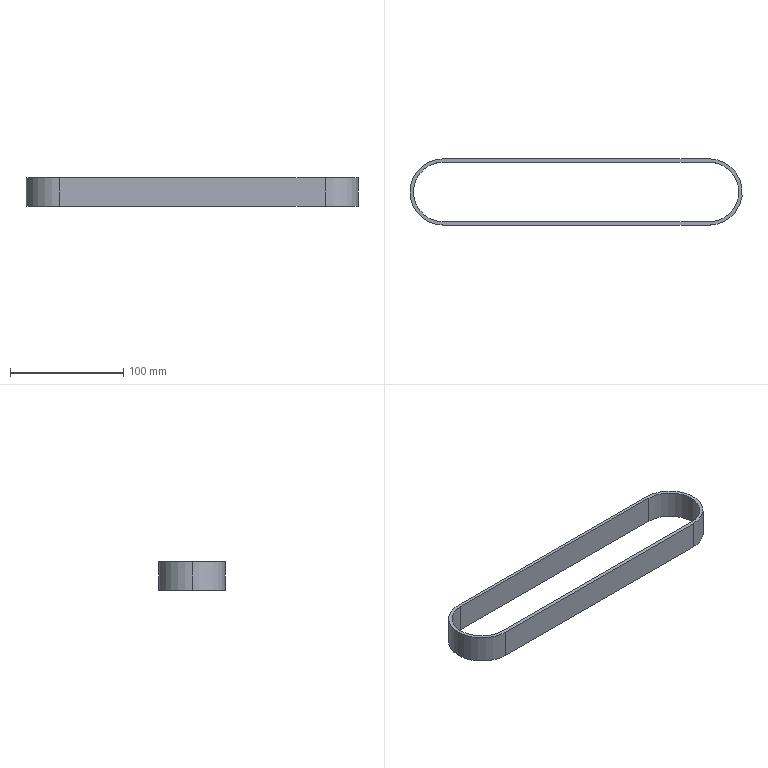Part | SolidWorks | features BeltProfileFeature 1, ExtruThin 1 | 1 solid | 12 faces | box 293.56 x 58.56 x 25 mm | volume 48341 mm3 | cylinder 6 | plane 6 | commonest cylinder face diameters 52.56 x3 58.56 x3
STEP:
#1=CARTESIAN_POINT('',(-235.,26.28,12.5));
#2=VERTEX_POINT('',#1);
#3=CARTESIAN_POINT('',(-261.28,0.,12.5));
#4=VERTEX_POINT('',#3);
#5=CARTESIAN_POINT('',(-235.,0.,12.5));
#6=DIRECTION('',(0.,0.,1.));
#7=DIRECTION('',(-1.,0.,0.));
#8=AXIS2_PLACEMENT_3D('',#5,#6,#7);
#9=CIRCLE('',#8,26.28);
#10=EDGE_CURVE('',#2,#4,#9,.T.);
#11=ORIENTED_EDGE('',*,*,#10,.T.);
#12=CARTESIAN_POINT('',(-261.28,0.,-12.5));
#13=VERTEX_POINT('',#12);
#14=CARTESIAN_POINT('',(-261.28,0.,12.5));
#15=DIRECTION('',(0.,0.,-1.));
#16=VECTOR('',#15,1000.);
#17=LINE('',#14,#16);
#18=EDGE_CURVE('',#4,#13,#17,.T.);
#19=ORIENTED_EDGE('',*,*,#18,.T.);
#20=CARTESIAN_POINT('',(-235.,26.28,-12.5));
#21=VERTEX_POINT('',#20);
#22=CARTESIAN_POINT('',(-235.,0.,-12.5));
#23=DIRECTION('',(0.,0.,1.));
#24=DIRECTION('',(-1.,0.,0.));
#25=AXIS2_PLACEMENT_3D('',#22,#23,#24);
#26=CIRCLE('',#25,26.28);
#27=EDGE_CURVE('',#21,#13,#26,.T.);
#28=ORIENTED_EDGE('',*,*,#27,.F.);
#29=CARTESIAN_POINT('',(-235.,26.28,12.5));
#30=DIRECTION('',(0.,0.,-1.));
#31=VECTOR('',#30,1000.);
#32=LINE('',#29,#31);
#33=EDGE_CURVE('',#2,#21,#32,.T.);
#34=ORIENTED_EDGE('',*,*,#33,.F.);
#35=EDGE_LOOP('',(#11,#19,#28,#34));
#36=FACE_OUTER_BOUND('',#35,.T.);
#37=CARTESIAN_POINT('',(-235.,0.,12.5));
#38=DIRECTION('',(0.,0.,-1.));
#39=DIRECTION('',(-1.,0.,0.));
#40=AXIS2_PLACEMENT_3D('',#37,#38,#39);
#41=CYLINDRICAL_SURFACE('',#40,26.28);
#42=ADVANCED_FACE('',(#36),#41,.F.);
#43=CARTESIAN_POINT('',(-264.28,0.,12.5));
#44=VERTEX_POINT('',#43);
#45=CARTESIAN_POINT('',(-235.,-29.28,12.5));
#46=VERTEX_POINT('',#45);
#47=CARTESIAN_POINT('',(-235.,0.,12.5));
#48=DIRECTION('',(0.,0.,1.));
#49=DIRECTION('',(-1.,0.,0.));
#50=AXIS2_PLACEMENT_3D('',#47,#48,#49);
#51=CIRCLE('',#50,29.28);
#52=EDGE_CURVE('',#44,#46,#51,.T.);
#53=ORIENTED_EDGE('',*,*,#52,.F.);
#54=CARTESIAN_POINT('',(-264.28,0.,-12.5));
#55=VERTEX_POINT('',#54);
#56=CARTESIAN_POINT('',(-264.28,0.,12.5));
#57=DIRECTION('',(0.,0.,-1.));
#58=VECTOR('',#57,1000.);
#59=LINE('',#56,#58);
#60=EDGE_CURVE('',#44,#55,#59,.T.);
#61=ORIENTED_EDGE('',*,*,#60,.T.);
#62=CARTESIAN_POINT('',(-235.,-29.28,-12.5));
#63=VERTEX_POINT('',#62);
#64=CARTESIAN_POINT('',(-235.,0.,-12.5));
#65=DIRECTION('',(0.,0.,1.));
#66=DIRECTION('',(-1.,0.,0.));
#67=AXIS2_PLACEMENT_3D('',#64,#65,#66);
#68=CIRCLE('',#67,29.28);
#69=EDGE_CURVE('',#55,#63,#68,.T.);
#70=ORIENTED_EDGE('',*,*,#69,.T.);
#71=CARTESIAN_POINT('',(-235.,-29.28,12.5));
#72=DIRECTION('',(0.,0.,-1.));
#73=VECTOR('',#72,1000.);
#74=LINE('',#71,#73);
#75=EDGE_CURVE('',#46,#63,#74,.T.);
#76=ORIENTED_EDGE('',*,*,#75,.F.);
#77=EDGE_LOOP('',(#53,#61,#70,#76));
#78=FACE_OUTER_BOUND('',#77,.T.);
#79=CARTESIAN_POINT('',(-235.,0.,12.5));
#80=DIRECTION('',(0.,0.,-1.));
#81=DIRECTION('',(-1.,0.,0.));
#82=AXIS2_PLACEMENT_3D('',#79,#80,#81);
#83=CYLINDRICAL_SURFACE('',#82,29.28);
#84=ADVANCED_FACE('',(#78),#83,.T.);
#85=CARTESIAN_POINT('',(0.,-29.28,12.5));
#86=VERTEX_POINT('',#85);
#87=CARTESIAN_POINT('',(0.,29.28,12.5));
#88=VERTEX_POINT('',#87);
#89=CARTESIAN_POINT('',(0.,0.,12.5));
#90=DIRECTION('',(0.,0.,1.));
#91=DIRECTION('',(-1.,0.,0.));
#92=AXIS2_PLACEMENT_3D('',#89,#90,#91);
#93=CIRCLE('',#92,29.28);
#94=EDGE_CURVE('',#86,#88,#93,.T.);
#95=ORIENTED_EDGE('',*,*,#94,.T.);
#96=CARTESIAN_POINT('',(-235.,29.28,12.5));
#97=VERTEX_POINT('',#96);
#98=CARTESIAN_POINT('',(0.,29.28,12.5));
#99=DIRECTION('',(-1.,0.,0.));
#100=VECTOR('',#99,1000.);
#101=LINE('',#98,#100);
#102=EDGE_CURVE('',#88,#97,#101,.T.);
#103=ORIENTED_EDGE('',*,*,#102,.T.);
#104=CARTESIAN_POINT('',(-235.,0.,12.5));
#105=DIRECTION('',(0.,0.,1.));
#106=DIRECTION('',(-1.,0.,0.));
#107=AXIS2_PLACEMENT_3D('',#104,#105,#106);
#108=CIRCLE('',#107,29.28);
#109=EDGE_CURVE('',#97,#44,#108,.T.);
#110=ORIENTED_EDGE('',*,*,#109,.T.);
#111=ORIENTED_EDGE('',*,*,#52,.T.);
#112=CARTESIAN_POINT('',(0.,-29.28,12.5));
#113=DIRECTION('',(1.,0.,0.));
#114=VECTOR('',#113,1000.);
#115=LINE('',#112,#114);
#116=EDGE_CURVE('',#46,#86,#115,.T.);
#117=ORIENTED_EDGE('',*,*,#116,.T.);
#118=EDGE_LOOP('',(#95,#103,#110,#111,#117));
#119=FACE_OUTER_BOUND('',#118,.T.);
#120=CARTESIAN_POINT('',(0.,-26.28,12.5));
#121=VERTEX_POINT('',#120);
#122=CARTESIAN_POINT('',(0.,26.28,12.5));
#123=VERTEX_POINT('',#122);
#124=CARTESIAN_POINT('',(0.,0.,12.5));
#125=DIRECTION('',(0.,0.,1.));
#126=DIRECTION('',(-1.,0.,0.));
#127=AXIS2_PLACEMENT_3D('',#124,#125,#126);
#128=CIRCLE('',#127,26.28);
#129=EDGE_CURVE('',#121,#123,#128,.T.);
#130=ORIENTED_EDGE('',*,*,#129,.F.);
#131=CARTESIAN_POINT('',(-235.,-26.28,12.5));
#132=VERTEX_POINT('',#131);
#133=CARTESIAN_POINT('',(0.,-26.28,12.5));
#134=DIRECTION('',(1.,0.,0.));
#135=VECTOR('',#134,1000.);
#136=LINE('',#133,#135);
#137=EDGE_CURVE('',#132,#121,#136,.T.);
#138=ORIENTED_EDGE('',*,*,#137,.F.);
#139=CARTESIAN_POINT('',(-235.,0.,12.5));
#140=DIRECTION('',(0.,0.,1.));
#141=DIRECTION('',(-1.,0.,0.));
#142=AXIS2_PLACEMENT_3D('',#139,#140,#141);
#143=CIRCLE('',#142,26.28);
#144=EDGE_CURVE('',#4,#132,#143,.T.);
#145=ORIENTED_EDGE('',*,*,#144,.F.);
#146=ORIENTED_EDGE('',*,*,#10,.F.);
#147=CARTESIAN_POINT('',(-235.,26.28,12.5));
#148=DIRECTION('',(-1.,0.,0.));
#149=VECTOR('',#148,1000.);
#150=LINE('',#147,#149);
#151=EDGE_CURVE('',#123,#2,#150,.T.);
#152=ORIENTED_EDGE('',*,*,#151,.F.);
#153=EDGE_LOOP('',(#130,#138,#145,#146,#152));
#154=FACE_BOUND('',#153,.T.);
#155=CARTESIAN_POINT('',(0.,0.,12.5));
#156=DIRECTION('',(0.,0.,-1.));
#157=DIRECTION('',(-1.,0.,0.));
#158=AXIS2_PLACEMENT_3D('',#155,#156,#157);
#159=PLANE('',#158);
#160=ADVANCED_FACE('',(#119,#154),#159,.F.);
#161=CARTESIAN_POINT('',(0.,-29.28,-12.5));
#162=VERTEX_POINT('',#161);
#163=CARTESIAN_POINT('',(0.,29.28,-12.5));
#164=VERTEX_POINT('',#163);
#165=CARTESIAN_POINT('',(0.,0.,-12.5));
#166=DIRECTION('',(0.,0.,1.));
#167=DIRECTION('',(-1.,0.,0.));
#168=AXIS2_PLACEMENT_3D('',#165,#166,#167);
#169=CIRCLE('',#168,29.28);
#170=EDGE_CURVE('',#162,#164,#169,.T.);
#171=ORIENTED_EDGE('',*,*,#170,.F.);
#172=CARTESIAN_POINT('',(0.,-29.28,-12.5));
#173=DIRECTION('',(1.,0.,0.));
#174=VECTOR('',#173,1000.);
#175=LINE('',#172,#174);
#176=EDGE_CURVE('',#63,#162,#175,.T.);
#177=ORIENTED_EDGE('',*,*,#176,.F.);
#178=ORIENTED_EDGE('',*,*,#69,.F.);
#179=CARTESIAN_POINT('',(-235.,29.28,-12.5));
#180=VERTEX_POINT('',#179);
#181=CARTESIAN_POINT('',(-235.,0.,-12.5));
#182=DIRECTION('',(0.,0.,1.));
#183=DIRECTION('',(-1.,0.,0.));
#184=AXIS2_PLACEMENT_3D('',#181,#182,#183);
#185=CIRCLE('',#184,29.28);
#186=EDGE_CURVE('',#180,#55,#185,.T.);
#187=ORIENTED_EDGE('',*,*,#186,.F.);
#188=CARTESIAN_POINT('',(0.,29.28,-12.5));
#189=DIRECTION('',(-1.,0.,0.));
#190=VECTOR('',#189,1000.);
#191=LINE('',#188,#190);
#192=EDGE_CURVE('',#164,#180,#191,.T.);
#193=ORIENTED_EDGE('',*,*,#192,.F.);
#194=EDGE_LOOP('',(#171,#177,#178,#187,#193));
#195=FACE_OUTER_BOUND('',#194,.T.);
#196=CARTESIAN_POINT('',(-235.,-26.28,-12.5));
#197=VERTEX_POINT('',#196);
#198=CARTESIAN_POINT('',(0.,-26.28,-12.5));
#199=VERTEX_POINT('',#198);
#200=CARTESIAN_POINT('',(0.,-26.28,-12.5));
#201=DIRECTION('',(1.,0.,0.));
#202=VECTOR('',#201,1000.);
#203=LINE('',#200,#202);
#204=EDGE_CURVE('',#197,#199,#203,.T.);
#205=ORIENTED_EDGE('',*,*,#204,.T.);
#206=CARTESIAN_POINT('',(0.,26.28,-12.5));
#207=VERTEX_POINT('',#206);
#208=CARTESIAN_POINT('',(0.,0.,-12.5));
#209=DIRECTION('',(0.,0.,1.));
#210=DIRECTION('',(-1.,0.,0.));
#211=AXIS2_PLACEMENT_3D('',#208,#209,#210);
#212=CIRCLE('',#211,26.28);
#213=EDGE_CURVE('',#199,#207,#212,.T.);
#214=ORIENTED_EDGE('',*,*,#213,.T.);
#215=CARTESIAN_POINT('',(-235.,26.28,-12.5));
#216=DIRECTION('',(-1.,0.,0.));
#217=VECTOR('',#216,1000.);
#218=LINE('',#215,#217);
#219=EDGE_CURVE('',#207,#21,#218,.T.);
#220=ORIENTED_EDGE('',*,*,#219,.T.);
#221=ORIENTED_EDGE('',*,*,#27,.T.);
#222=CARTESIAN_POINT('',(-235.,0.,-12.5));
#223=DIRECTION('',(0.,0.,1.));
#224=DIRECTION('',(-1.,0.,0.));
#225=AXIS2_PLACEMENT_3D('',#222,#223,#224);
#226=CIRCLE('',#225,26.28);
#227=EDGE_CURVE('',#13,#197,#226,.T.);
#228=ORIENTED_EDGE('',*,*,#227,.T.);
#229=EDGE_LOOP('',(#205,#214,#220,#221,#228));
#230=FACE_BOUND('',#229,.T.);
#231=CARTESIAN_POINT('',(0.,0.,-12.5));
#232=DIRECTION('',(0.,0.,-1.));
#233=DIRECTION('',(-1.,0.,0.));
#234=AXIS2_PLACEMENT_3D('',#231,#232,#233);
#235=PLANE('',#234);
#236=ADVANCED_FACE('',(#195,#230),#235,.T.);
#237=ORIENTED_EDGE('',*,*,#170,.T.);
#238=CARTESIAN_POINT('',(0.,29.28,12.5));
#239=DIRECTION('',(0.,0.,-1.));
#240=VECTOR('',#239,1000.);
#241=LINE('',#238,#240);
#242=EDGE_CURVE('',#88,#164,#241,.T.);
#243=ORIENTED_EDGE('',*,*,#242,.F.);
#244=ORIENTED_EDGE('',*,*,#94,.F.);
#245=CARTESIAN_POINT('',(0.,-29.28,12.5));
#246=DIRECTION('',(0.,0.,-1.));
#247=VECTOR('',#246,1000.);
#248=LINE('',#245,#247);
#249=EDGE_CURVE('',#86,#162,#248,.T.);
#250=ORIENTED_EDGE('',*,*,#249,.T.);
#251=EDGE_LOOP('',(#237,#243,#244,#250));
#252=FACE_OUTER_BOUND('',#251,.T.);
#253=CARTESIAN_POINT('',(0.,0.,12.5));
#254=DIRECTION('',(0.,0.,-1.));
#255=DIRECTION('',(-1.,0.,0.));
#256=AXIS2_PLACEMENT_3D('',#253,#254,#255);
#257=CYLINDRICAL_SURFACE('',#256,29.28);
#258=ADVANCED_FACE('',(#252),#257,.T.);
#259=ORIENTED_EDGE('',*,*,#192,.T.);
#260=CARTESIAN_POINT('',(-235.,29.28,12.5));
#261=DIRECTION('',(0.,0.,-1.));
#262=VECTOR('',#261,1000.);
#263=LINE('',#260,#262);
#264=EDGE_CURVE('',#97,#180,#263,.T.);
#265=ORIENTED_EDGE('',*,*,#264,.F.);
#266=ORIENTED_EDGE('',*,*,#102,.F.);
#267=ORIENTED_EDGE('',*,*,#242,.T.);
#268=EDGE_LOOP('',(#259,#265,#266,#267));
#269=FACE_OUTER_BOUND('',#268,.T.);
#270=CARTESIAN_POINT('',(0.,29.28,12.5));
#271=DIRECTION('',(0.,-1.,0.));
#272=DIRECTION('',(0.,0.,-1.));
#273=AXIS2_PLACEMENT_3D('',#270,#271,#272);
#274=PLANE('',#273);
#275=ADVANCED_FACE('',(#269),#274,.F.);
#276=ORIENTED_EDGE('',*,*,#60,.F.);
#277=ORIENTED_EDGE('',*,*,#109,.F.);
#278=ORIENTED_EDGE('',*,*,#264,.T.);
#279=ORIENTED_EDGE('',*,*,#186,.T.);
#280=EDGE_LOOP('',(#276,#277,#278,#279));
#281=FACE_OUTER_BOUND('',#280,.T.);
#282=CARTESIAN_POINT('',(-235.,0.,12.5));
#283=DIRECTION('',(0.,0.,-1.));
#284=DIRECTION('',(-1.,0.,0.));
#285=AXIS2_PLACEMENT_3D('',#282,#283,#284);
#286=CYLINDRICAL_SURFACE('',#285,29.28);
#287=ADVANCED_FACE('',(#281),#286,.T.);
#288=ORIENTED_EDGE('',*,*,#176,.T.);
#289=ORIENTED_EDGE('',*,*,#249,.F.);
#290=ORIENTED_EDGE('',*,*,#116,.F.);
#291=ORIENTED_EDGE('',*,*,#75,.T.);
#292=EDGE_LOOP('',(#288,#289,#290,#291));
#293=FACE_OUTER_BOUND('',#292,.T.);
#294=CARTESIAN_POINT('',(0.,-29.28,12.5));
#295=DIRECTION('',(0.,1.,0.));
#296=DIRECTION('',(0.,0.,1.));
#297=AXIS2_PLACEMENT_3D('',#294,#295,#296);
#298=PLANE('',#297);
#299=ADVANCED_FACE('',(#293),#298,.F.);
#300=ORIENTED_EDGE('',*,*,#213,.F.);
#301=CARTESIAN_POINT('',(0.,-26.28,12.5));
#302=DIRECTION('',(0.,0.,-1.));
#303=VECTOR('',#302,1000.);
#304=LINE('',#301,#303);
#305=EDGE_CURVE('',#121,#199,#304,.T.);
#306=ORIENTED_EDGE('',*,*,#305,.F.);
#307=ORIENTED_EDGE('',*,*,#129,.T.);
#308=CARTESIAN_POINT('',(0.,26.28,12.5));
#309=DIRECTION('',(0.,0.,-1.));
#310=VECTOR('',#309,1000.);
#311=LINE('',#308,#310);
#312=EDGE_CURVE('',#123,#207,#311,.T.);
#313=ORIENTED_EDGE('',*,*,#312,.T.);
#314=EDGE_LOOP('',(#300,#306,#307,#313));
#315=FACE_OUTER_BOUND('',#314,.T.);
#316=CARTESIAN_POINT('',(0.,0.,12.5));
#317=DIRECTION('',(0.,0.,-1.));
#318=DIRECTION('',(-1.,0.,0.));
#319=AXIS2_PLACEMENT_3D('',#316,#317,#318);
#320=CYLINDRICAL_SURFACE('',#319,26.28);
#321=ADVANCED_FACE('',(#315),#320,.F.);
#322=ORIENTED_EDGE('',*,*,#219,.F.);
#323=ORIENTED_EDGE('',*,*,#312,.F.);
#324=ORIENTED_EDGE('',*,*,#151,.T.);
#325=ORIENTED_EDGE('',*,*,#33,.T.);
#326=EDGE_LOOP('',(#322,#323,#324,#325));
#327=FACE_OUTER_BOUND('',#326,.T.);
#328=CARTESIAN_POINT('',(-235.,26.28,12.5));
#329=DIRECTION('',(0.,-1.,0.));
#330=DIRECTION('',(0.,0.,-1.));
#331=AXIS2_PLACEMENT_3D('',#328,#329,#330);
#332=PLANE('',#331);
#333=ADVANCED_FACE('',(#327),#332,.T.);
#334=ORIENTED_EDGE('',*,*,#18,.F.);
#335=ORIENTED_EDGE('',*,*,#144,.T.);
#336=CARTESIAN_POINT('',(-235.,-26.28,12.5));
#337=DIRECTION('',(0.,0.,-1.));
#338=VECTOR('',#337,1000.);
#339=LINE('',#336,#338);
#340=EDGE_CURVE('',#132,#197,#339,.T.);
#341=ORIENTED_EDGE('',*,*,#340,.T.);
#342=ORIENTED_EDGE('',*,*,#227,.F.);
#343=EDGE_LOOP('',(#334,#335,#341,#342));
#344=FACE_OUTER_BOUND('',#343,.T.);
#345=CARTESIAN_POINT('',(-235.,0.,12.5));
#346=DIRECTION('',(0.,0.,-1.));
#347=DIRECTION('',(-1.,0.,0.));
#348=AXIS2_PLACEMENT_3D('',#345,#346,#347);
#349=CYLINDRICAL_SURFACE('',#348,26.28);
#350=ADVANCED_FACE('',(#344),#349,.F.);
#351=ORIENTED_EDGE('',*,*,#204,.F.);
#352=ORIENTED_EDGE('',*,*,#340,.F.);
#353=ORIENTED_EDGE('',*,*,#137,.T.);
#354=ORIENTED_EDGE('',*,*,#305,.T.);
#355=EDGE_LOOP('',(#351,#352,#353,#354));
#356=FACE_OUTER_BOUND('',#355,.T.);
#357=CARTESIAN_POINT('',(0.,-26.28,12.5));
#358=DIRECTION('',(0.,1.,0.));
#359=DIRECTION('',(0.,0.,1.));
#360=AXIS2_PLACEMENT_3D('',#357,#358,#359);
#361=PLANE('',#360);
#362=ADVANCED_FACE('',(#356),#361,.T.);
#363=CLOSED_SHELL('',(#42,#84,#160,#236,#258,#275,#287,#299,#321,#333,#350,#362));
#364=MANIFOLD_SOLID_BREP('',#363);
#365=CARTESIAN_POINT('',(0.,0.,0.));
#366=DIRECTION('',(0.,0.,1.));
#367=DIRECTION('',(1.,0.,0.));
#368=AXIS2_PLACEMENT_3D('',#365,#366,#367);
#369=(LENGTH_UNIT()NAMED_UNIT(*)SI_UNIT(.MILLI.,.METRE.));
#370=UNCERTAINTY_MEASURE_WITH_UNIT(LENGTH_MEASURE(0.00001),#369,'','');
#371=(NAMED_UNIT(*)PLANE_ANGLE_UNIT()SI_UNIT($,.RADIAN.));
#372=(NAMED_UNIT(*)SI_UNIT($,.STERADIAN.)SOLID_ANGLE_UNIT());
#373=(GEOMETRIC_REPRESENTATION_CONTEXT(3)GLOBAL_UNCERTAINTY_ASSIGNED_CONTEXT((#370))GLOBAL_UNIT_ASSIGNED_CONTEXT((#369,#371,#372))REPRESENTATION_CONTEXT('',''));
#374=ADVANCED_BREP_SHAPE_REPRESENTATION('',(#364,#368),#373);